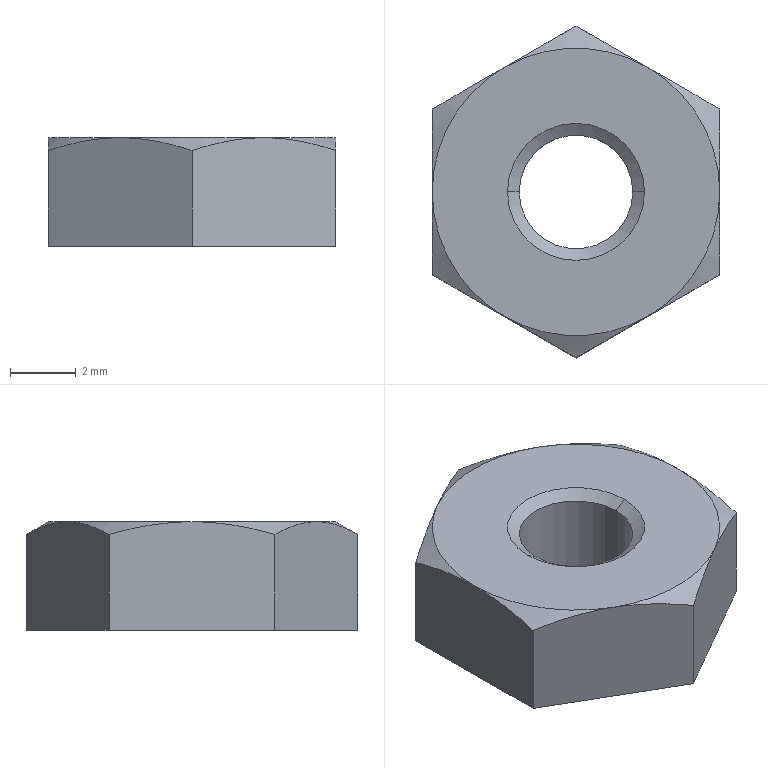Part | SolidWorks | features BaseBody 1 | 1 solid | 22 faces | box 8.738 x 10.089 x 3.302 mm | volume 185.504 mm3 | cone 10 | plane 8 | cylinder 4 | commonest cylinder face diameters 3.454 x2 4.166 x2
STEP:
#1=CARTESIAN_POINT('',(0.,-2.083,-3.302));
#2=VERTEX_POINT('',#1);
#3=CARTESIAN_POINT('',(0.,2.083,-3.302));
#4=VERTEX_POINT('',#3);
#5=CARTESIAN_POINT('',(0.,0.,-3.302));
#6=DIRECTION('',(0.,0.,-1.));
#7=DIRECTION('',(0.,-1.,0.));
#8=AXIS2_PLACEMENT_3D('',#5,#6,#7);
#9=CIRCLE('',#8,2.083);
#10=EDGE_CURVE('',#2,#4,#9,.T.);
#11=ORIENTED_EDGE('',*,*,#10,.T.);
#12=CARTESIAN_POINT('',(0.,2.083,-3.277));
#13=VERTEX_POINT('',#12);
#14=CARTESIAN_POINT('',(0.,2.083,-3.302));
#15=DIRECTION('',(0.,0.,1.));
#16=VECTOR('',#15,1000.);
#17=LINE('',#14,#16);
#18=EDGE_CURVE('',#4,#13,#17,.T.);
#19=ORIENTED_EDGE('',*,*,#18,.T.);
#20=CARTESIAN_POINT('',(-2.083,0.,-3.277));
#21=VERTEX_POINT('',#20);
#22=CARTESIAN_POINT('',(0.,0.,-3.277));
#23=DIRECTION('',(0.,0.,1.));
#24=DIRECTION('',(1.,0.,0.));
#25=AXIS2_PLACEMENT_3D('',#22,#23,#24);
#26=CIRCLE('',#25,2.083);
#27=EDGE_CURVE('',#13,#21,#26,.T.);
#28=ORIENTED_EDGE('',*,*,#27,.T.);
#29=CARTESIAN_POINT('',(0.,-2.083,-3.277));
#30=VERTEX_POINT('',#29);
#31=CARTESIAN_POINT('',(0.,0.,-3.277));
#32=DIRECTION('',(0.,0.,1.));
#33=DIRECTION('',(1.,0.,0.));
#34=AXIS2_PLACEMENT_3D('',#31,#32,#33);
#35=CIRCLE('',#34,2.083);
#36=EDGE_CURVE('',#21,#30,#35,.T.);
#37=ORIENTED_EDGE('',*,*,#36,.T.);
#38=CARTESIAN_POINT('',(0.,-2.083,-3.302));
#39=DIRECTION('',(0.,0.,1.));
#40=VECTOR('',#39,1000.);
#41=LINE('',#38,#40);
#42=EDGE_CURVE('',#2,#30,#41,.T.);
#43=ORIENTED_EDGE('',*,*,#42,.F.);
#44=EDGE_LOOP('',(#11,#19,#28,#37,#43));
#45=FACE_OUTER_BOUND('',#44,.T.);
#46=CARTESIAN_POINT('',(0.,0.,-3.302));
#47=DIRECTION('',(0.,0.,1.));
#48=DIRECTION('',(0.,-1.,0.));
#49=AXIS2_PLACEMENT_3D('',#46,#47,#48);
#50=CYLINDRICAL_SURFACE('',#49,2.083);
#51=ADVANCED_FACE('',(#45),#50,.F.);
#52=CARTESIAN_POINT('',(-1.727,0.,-3.028));
#53=VERTEX_POINT('',#52);
#54=CARTESIAN_POINT('',(1.727,0.,-3.028));
#55=VERTEX_POINT('',#54);
#56=CARTESIAN_POINT('',(0.,0.,-3.028));
#57=DIRECTION('',(0.,0.,1.));
#58=DIRECTION('',(-1.,0.,0.));
#59=AXIS2_PLACEMENT_3D('',#56,#57,#58);
#60=CIRCLE('',#59,1.727);
#61=EDGE_CURVE('',#53,#55,#60,.T.);
#62=ORIENTED_EDGE('',*,*,#61,.T.);
#63=CARTESIAN_POINT('',(2.083,0.,-3.277));
#64=VERTEX_POINT('',#63);
#65=CARTESIAN_POINT('',(1.727,0.,-3.028));
#66=DIRECTION('',(0.8192,0.,-0.5736));
#67=VECTOR('',#66,1000.);
#68=LINE('',#65,#67);
#69=EDGE_CURVE('',#55,#64,#68,.T.);
#70=ORIENTED_EDGE('',*,*,#69,.T.);
#71=CARTESIAN_POINT('',(0.,0.,-3.277));
#72=DIRECTION('',(0.,0.,1.));
#73=DIRECTION('',(1.,0.,0.));
#74=AXIS2_PLACEMENT_3D('',#71,#72,#73);
#75=CIRCLE('',#74,2.083);
#76=EDGE_CURVE('',#30,#64,#75,.T.);
#77=ORIENTED_EDGE('',*,*,#76,.F.);
#78=ORIENTED_EDGE('',*,*,#36,.F.);
#79=CARTESIAN_POINT('',(-1.727,0.,-3.028));
#80=DIRECTION('',(-0.8192,0.,-0.5736));
#81=VECTOR('',#80,1000.);
#82=LINE('',#79,#81);
#83=EDGE_CURVE('',#53,#21,#82,.T.);
#84=ORIENTED_EDGE('',*,*,#83,.F.);
#85=EDGE_LOOP('',(#62,#70,#77,#78,#84));
#86=FACE_OUTER_BOUND('',#85,.T.);
#87=CARTESIAN_POINT('',(0.,0.,-3.028));
#88=DIRECTION('',(0.,0.,-1.));
#89=DIRECTION('',(-1.,0.,0.));
#90=AXIS2_PLACEMENT_3D('',#87,#88,#89);
#91=CONICAL_SURFACE('',#90,1.727,0.9599);
#92=ADVANCED_FACE('',(#86),#91,.F.);
#93=ORIENTED_EDGE('',*,*,#61,.F.);
#94=CARTESIAN_POINT('',(-1.727,0.,-0.249));
#95=VERTEX_POINT('',#94);
#96=CARTESIAN_POINT('',(-1.727,0.,-3.028));
#97=DIRECTION('',(0.,0.,1.));
#98=VECTOR('',#97,1000.);
#99=LINE('',#96,#98);
#100=EDGE_CURVE('',#53,#95,#99,.T.);
#101=ORIENTED_EDGE('',*,*,#100,.T.);
#102=CARTESIAN_POINT('',(1.727,0.,-0.249));
#103=VERTEX_POINT('',#102);
#104=CARTESIAN_POINT('',(0.,0.,-0.249));
#105=DIRECTION('',(0.,0.,1.));
#106=DIRECTION('',(1.,0.,0.));
#107=AXIS2_PLACEMENT_3D('',#104,#105,#106);
#108=CIRCLE('',#107,1.727);
#109=EDGE_CURVE('',#95,#103,#108,.T.);
#110=ORIENTED_EDGE('',*,*,#109,.T.);
#111=CARTESIAN_POINT('',(1.727,0.,-3.028));
#112=DIRECTION('',(0.,0.,1.));
#113=VECTOR('',#112,1000.);
#114=LINE('',#111,#113);
#115=EDGE_CURVE('',#55,#103,#114,.T.);
#116=ORIENTED_EDGE('',*,*,#115,.F.);
#117=EDGE_LOOP('',(#93,#101,#110,#116));
#118=FACE_OUTER_BOUND('',#117,.T.);
#119=CARTESIAN_POINT('',(0.,0.,-3.028));
#120=DIRECTION('',(0.,0.,1.));
#121=DIRECTION('',(1.,0.,0.));
#122=AXIS2_PLACEMENT_3D('',#119,#120,#121);
#123=CYLINDRICAL_SURFACE('',#122,1.727);
#124=ADVANCED_FACE('',(#118),#123,.F.);
#125=ORIENTED_EDGE('',*,*,#109,.F.);
#126=CARTESIAN_POINT('',(-2.083,0.,0.));
#127=VERTEX_POINT('',#126);
#128=CARTESIAN_POINT('',(-1.727,0.,-0.249));
#129=DIRECTION('',(-0.8192,0.,0.5736));
#130=VECTOR('',#129,1000.);
#131=LINE('',#128,#130);
#132=EDGE_CURVE('',#95,#127,#131,.T.);
#133=ORIENTED_EDGE('',*,*,#132,.T.);
#134=CARTESIAN_POINT('',(2.083,0.,0.));
#135=VERTEX_POINT('',#134);
#136=CARTESIAN_POINT('',(0.,0.,0.));
#137=DIRECTION('',(0.,0.,1.));
#138=DIRECTION('',(1.,0.,0.));
#139=AXIS2_PLACEMENT_3D('',#136,#137,#138);
#140=CIRCLE('',#139,2.083);
#141=EDGE_CURVE('',#127,#135,#140,.T.);
#142=ORIENTED_EDGE('',*,*,#141,.T.);
#143=CARTESIAN_POINT('',(1.727,0.,-0.249));
#144=DIRECTION('',(0.8192,0.,0.5736));
#145=VECTOR('',#144,1000.);
#146=LINE('',#143,#145);
#147=EDGE_CURVE('',#103,#135,#146,.T.);
#148=ORIENTED_EDGE('',*,*,#147,.F.);
#149=EDGE_LOOP('',(#125,#133,#142,#148));
#150=FACE_OUTER_BOUND('',#149,.T.);
#151=CARTESIAN_POINT('',(0.,0.,-0.249));
#152=DIRECTION('',(0.,0.,1.));
#153=DIRECTION('',(1.,0.,0.));
#154=AXIS2_PLACEMENT_3D('',#151,#152,#153);
#155=CONICAL_SURFACE('',#154,1.727,0.9599);
#156=ADVANCED_FACE('',(#150),#155,.F.);
#157=ORIENTED_EDGE('',*,*,#18,.F.);
#158=CARTESIAN_POINT('',(0.,0.,-3.302));
#159=DIRECTION('',(0.,0.,-1.));
#160=DIRECTION('',(0.,-1.,0.));
#161=AXIS2_PLACEMENT_3D('',#158,#159,#160);
#162=CIRCLE('',#161,2.083);
#163=EDGE_CURVE('',#4,#2,#162,.T.);
#164=ORIENTED_EDGE('',*,*,#163,.T.);
#165=ORIENTED_EDGE('',*,*,#42,.T.);
#166=ORIENTED_EDGE('',*,*,#76,.T.);
#167=CARTESIAN_POINT('',(0.,0.,-3.277));
#168=DIRECTION('',(0.,0.,1.));
#169=DIRECTION('',(1.,0.,0.));
#170=AXIS2_PLACEMENT_3D('',#167,#168,#169);
#171=CIRCLE('',#170,2.083);
#172=EDGE_CURVE('',#64,#13,#171,.T.);
#173=ORIENTED_EDGE('',*,*,#172,.T.);
#174=EDGE_LOOP('',(#157,#164,#165,#166,#173));
#175=FACE_OUTER_BOUND('',#174,.T.);
#176=CARTESIAN_POINT('',(0.,0.,-3.302));
#177=DIRECTION('',(0.,0.,1.));
#178=DIRECTION('',(0.,-1.,0.));
#179=AXIS2_PLACEMENT_3D('',#176,#177,#178);
#180=CYLINDRICAL_SURFACE('',#179,2.083);
#181=ADVANCED_FACE('',(#175),#180,.F.);
#182=ORIENTED_EDGE('',*,*,#69,.F.);
#183=CARTESIAN_POINT('',(0.,0.,-3.028));
#184=DIRECTION('',(0.,0.,1.));
#185=DIRECTION('',(-1.,0.,0.));
#186=AXIS2_PLACEMENT_3D('',#183,#184,#185);
#187=CIRCLE('',#186,1.727);
#188=EDGE_CURVE('',#55,#53,#187,.T.);
#189=ORIENTED_EDGE('',*,*,#188,.T.);
#190=ORIENTED_EDGE('',*,*,#83,.T.);
#191=ORIENTED_EDGE('',*,*,#27,.F.);
#192=ORIENTED_EDGE('',*,*,#172,.F.);
#193=EDGE_LOOP('',(#182,#189,#190,#191,#192));
#194=FACE_OUTER_BOUND('',#193,.T.);
#195=CARTESIAN_POINT('',(0.,0.,-3.028));
#196=DIRECTION('',(0.,0.,-1.));
#197=DIRECTION('',(-1.,0.,0.));
#198=AXIS2_PLACEMENT_3D('',#195,#196,#197);
#199=CONICAL_SURFACE('',#198,1.727,0.9599);
#200=ADVANCED_FACE('',(#194),#199,.F.);
#201=ORIENTED_EDGE('',*,*,#10,.F.);
#202=ORIENTED_EDGE('',*,*,#163,.F.);
#203=EDGE_LOOP('',(#201,#202));
#204=FACE_BOUND('',#203,.T.);
#205=CARTESIAN_POINT('',(0.,-5.045,-3.302));
#206=VERTEX_POINT('',#205);
#207=CARTESIAN_POINT('',(-4.369,-2.522,-3.302));
#208=VERTEX_POINT('',#207);
#209=CARTESIAN_POINT('',(0.,-5.045,-3.302));
#210=DIRECTION('',(-0.866,0.5,0.));
#211=VECTOR('',#210,1000.);
#212=LINE('',#209,#211);
#213=EDGE_CURVE('',#206,#208,#212,.T.);
#214=ORIENTED_EDGE('',*,*,#213,.T.);
#215=CARTESIAN_POINT('',(-4.369,2.522,-3.302));
#216=VERTEX_POINT('',#215);
#217=CARTESIAN_POINT('',(-4.369,0.,-3.302));
#218=DIRECTION('',(0.,1.,0.));
#219=VECTOR('',#218,1000.);
#220=LINE('',#217,#219);
#221=EDGE_CURVE('',#208,#216,#220,.T.);
#222=ORIENTED_EDGE('',*,*,#221,.T.);
#223=CARTESIAN_POINT('',(0.,5.045,-3.302));
#224=VERTEX_POINT('',#223);
#225=CARTESIAN_POINT('',(-4.369,2.522,-3.302));
#226=DIRECTION('',(0.866,0.5,0.));
#227=VECTOR('',#226,1000.);
#228=LINE('',#225,#227);
#229=EDGE_CURVE('',#216,#224,#228,.T.);
#230=ORIENTED_EDGE('',*,*,#229,.T.);
#231=CARTESIAN_POINT('',(4.369,2.522,-3.302));
#232=VERTEX_POINT('',#231);
#233=CARTESIAN_POINT('',(0.,5.045,-3.302));
#234=DIRECTION('',(0.866,-0.5,0.));
#235=VECTOR('',#234,1000.);
#236=LINE('',#233,#235);
#237=EDGE_CURVE('',#224,#232,#236,.T.);
#238=ORIENTED_EDGE('',*,*,#237,.T.);
#239=CARTESIAN_POINT('',(4.369,-2.522,-3.302));
#240=VERTEX_POINT('',#239);
#241=CARTESIAN_POINT('',(4.369,0.,-3.302));
#242=DIRECTION('',(0.,-1.,0.));
#243=VECTOR('',#242,1000.);
#244=LINE('',#241,#243);
#245=EDGE_CURVE('',#232,#240,#244,.T.);
#246=ORIENTED_EDGE('',*,*,#245,.T.);
#247=CARTESIAN_POINT('',(4.369,-2.522,-3.302));
#248=DIRECTION('',(-0.866,-0.5,0.));
#249=VECTOR('',#248,1000.);
#250=LINE('',#247,#249);
#251=EDGE_CURVE('',#240,#206,#250,.T.);
#252=ORIENTED_EDGE('',*,*,#251,.T.);
#253=EDGE_LOOP('',(#214,#222,#230,#238,#246,#252));
#254=FACE_OUTER_BOUND('',#253,.T.);
#255=CARTESIAN_POINT('',(4.369,-5.105,-3.302));
#256=DIRECTION('',(0.,0.,-1.));
#257=DIRECTION('',(-1.,0.,0.));
#258=AXIS2_PLACEMENT_3D('',#255,#256,#257);
#259=PLANE('',#258);
#260=ADVANCED_FACE('',(#204,#254),#259,.T.);
#261=ORIENTED_EDGE('',*,*,#100,.F.);
#262=ORIENTED_EDGE('',*,*,#188,.F.);
#263=ORIENTED_EDGE('',*,*,#115,.T.);
#264=CARTESIAN_POINT('',(0.,0.,-0.249));
#265=DIRECTION('',(0.,0.,1.));
#266=DIRECTION('',(1.,0.,0.));
#267=AXIS2_PLACEMENT_3D('',#264,#265,#266);
#268=CIRCLE('',#267,1.727);
#269=EDGE_CURVE('',#103,#95,#268,.T.);
#270=ORIENTED_EDGE('',*,*,#269,.T.);
#271=EDGE_LOOP('',(#261,#262,#263,#270));
#272=FACE_OUTER_BOUND('',#271,.T.);
#273=CARTESIAN_POINT('',(0.,0.,-3.028));
#274=DIRECTION('',(0.,0.,1.));
#275=DIRECTION('',(1.,0.,0.));
#276=AXIS2_PLACEMENT_3D('',#273,#274,#275);
#277=CYLINDRICAL_SURFACE('',#276,1.727);
#278=ADVANCED_FACE('',(#272),#277,.F.);
#279=CARTESIAN_POINT('',(-4.369,2.522,-0.3902));
#280=VERTEX_POINT('',#279);
#281=CARTESIAN_POINT('',(-4.369,2.522,-1.641));
#282=DIRECTION('',(0.,0.,-1.));
#283=VECTOR('',#282,1000.);
#284=LINE('',#281,#283);
#285=EDGE_CURVE('',#280,#216,#284,.T.);
#286=ORIENTED_EDGE('',*,*,#285,.T.);
#287=ORIENTED_EDGE('',*,*,#221,.F.);
#288=CARTESIAN_POINT('',(-4.369,-2.522,-0.3902));
#289=VERTEX_POINT('',#288);
#290=CARTESIAN_POINT('',(-4.369,-2.522,-1.641));
#291=DIRECTION('',(0.,0.,1.));
#292=VECTOR('',#291,1000.);
#293=LINE('',#290,#292);
#294=EDGE_CURVE('',#208,#289,#293,.T.);
#295=ORIENTED_EDGE('',*,*,#294,.T.);
#296=CARTESIAN_POINT('',(-4.369,0.,0.));
#297=VERTEX_POINT('',#296);
#298=CARTESIAN_POINT('',(-4.369,-2.522,-0.3902));
#299=CARTESIAN_POINT('',(-4.369,-1.698,-0.1523));
#300=CARTESIAN_POINT('',(-4.369,-0.8609,0.));
#301=CARTESIAN_POINT('',(-4.369,0.,0.));
#302=B_SPLINE_CURVE_WITH_KNOTS('',3,(#298,#299,#300,#301),.UNSPECIFIED.,.F.,.F.,(4,4),(0.,0.002552),.UNSPECIFIED.);
#303=EDGE_CURVE('',#289,#297,#302,.T.);
#304=ORIENTED_EDGE('',*,*,#303,.T.);
#305=CARTESIAN_POINT('',(-4.369,0.,0.));
#306=CARTESIAN_POINT('',(-4.369,0.8609,0.));
#307=CARTESIAN_POINT('',(-4.369,1.698,-0.1523));
#308=CARTESIAN_POINT('',(-4.369,2.522,-0.3902));
#309=B_SPLINE_CURVE_WITH_KNOTS('',3,(#305,#306,#307,#308),.UNSPECIFIED.,.F.,.F.,(4,4),(0.,0.002552),.UNSPECIFIED.);
#310=EDGE_CURVE('',#297,#280,#309,.T.);
#311=ORIENTED_EDGE('',*,*,#310,.T.);
#312=EDGE_LOOP('',(#286,#287,#295,#304,#311));
#313=FACE_OUTER_BOUND('',#312,.T.);
#314=CARTESIAN_POINT('',(-4.369,-2.522,-3.302));
#315=DIRECTION('',(-1.,0.,0.));
#316=DIRECTION('',(0.,0.,1.));
#317=AXIS2_PLACEMENT_3D('',#314,#315,#316);
#318=PLANE('',#317);
#319=ADVANCED_FACE('',(#313),#318,.T.);
#320=ORIENTED_EDGE('',*,*,#294,.F.);
#321=ORIENTED_EDGE('',*,*,#213,.F.);
#322=CARTESIAN_POINT('',(0.,-5.045,-0.3902));
#323=VERTEX_POINT('',#322);
#324=CARTESIAN_POINT('',(0.,-5.045,-1.641));
#325=DIRECTION('',(0.,0.,1.));
#326=VECTOR('',#325,1000.);
#327=LINE('',#324,#326);
#328=EDGE_CURVE('',#206,#323,#327,.T.);
#329=ORIENTED_EDGE('',*,*,#328,.T.);
#330=CARTESIAN_POINT('',(-2.184,-3.783,0.));
#331=VERTEX_POINT('',#330);
#332=CARTESIAN_POINT('',(0.,-5.045,-0.3902));
#333=CARTESIAN_POINT('',(-0.7137,-4.633,-0.1523));
#334=CARTESIAN_POINT('',(-1.439,-4.214,0.));
#335=CARTESIAN_POINT('',(-2.184,-3.783,0.));
#336=B_SPLINE_CURVE_WITH_KNOTS('',3,(#332,#333,#334,#335),.UNSPECIFIED.,.F.,.F.,(4,4),(0.,0.002552),.UNSPECIFIED.);
#337=EDGE_CURVE('',#323,#331,#336,.T.);
#338=ORIENTED_EDGE('',*,*,#337,.T.);
#339=CARTESIAN_POINT('',(-2.184,-3.783,0.));
#340=CARTESIAN_POINT('',(-2.93,-3.353,0.));
#341=CARTESIAN_POINT('',(-3.655,-2.934,-0.1523));
#342=CARTESIAN_POINT('',(-4.369,-2.522,-0.3902));
#343=B_SPLINE_CURVE_WITH_KNOTS('',3,(#339,#340,#341,#342),.UNSPECIFIED.,.F.,.F.,(4,4),(0.,0.002552),.UNSPECIFIED.);
#344=EDGE_CURVE('',#331,#289,#343,.T.);
#345=ORIENTED_EDGE('',*,*,#344,.T.);
#346=EDGE_LOOP('',(#320,#321,#329,#338,#345));
#347=FACE_OUTER_BOUND('',#346,.T.);
#348=CARTESIAN_POINT('',(-4.369,-2.522,-3.302));
#349=DIRECTION('',(-0.5,-0.866,0.));
#350=DIRECTION('',(0.866,-0.5,0.));
#351=AXIS2_PLACEMENT_3D('',#348,#349,#350);
#352=PLANE('',#351);
#353=ADVANCED_FACE('',(#347),#352,.T.);
#354=ORIENTED_EDGE('',*,*,#328,.F.);
#355=ORIENTED_EDGE('',*,*,#251,.F.);
#356=CARTESIAN_POINT('',(4.369,-2.522,-0.3902));
#357=VERTEX_POINT('',#356);
#358=CARTESIAN_POINT('',(4.369,-2.522,-1.641));
#359=DIRECTION('',(0.,0.,1.));
#360=VECTOR('',#359,1000.);
#361=LINE('',#358,#360);
#362=EDGE_CURVE('',#240,#357,#361,.T.);
#363=ORIENTED_EDGE('',*,*,#362,.T.);
#364=CARTESIAN_POINT('',(2.184,-3.783,0.));
#365=VERTEX_POINT('',#364);
#366=CARTESIAN_POINT('',(4.369,-2.522,-0.3902));
#367=CARTESIAN_POINT('',(3.655,-2.934,-0.1523));
#368=CARTESIAN_POINT('',(2.93,-3.353,0.));
#369=CARTESIAN_POINT('',(2.184,-3.783,0.));
#370=B_SPLINE_CURVE_WITH_KNOTS('',3,(#366,#367,#368,#369),.UNSPECIFIED.,.F.,.F.,(4,4),(0.,0.002552),.UNSPECIFIED.);
#371=EDGE_CURVE('',#357,#365,#370,.T.);
#372=ORIENTED_EDGE('',*,*,#371,.T.);
#373=CARTESIAN_POINT('',(2.184,-3.783,0.));
#374=CARTESIAN_POINT('',(1.439,-4.214,0.));
#375=CARTESIAN_POINT('',(0.7137,-4.633,-0.1523));
#376=CARTESIAN_POINT('',(0.,-5.045,-0.3902));
#377=B_SPLINE_CURVE_WITH_KNOTS('',3,(#373,#374,#375,#376),.UNSPECIFIED.,.F.,.F.,(4,4),(0.,0.002552),.UNSPECIFIED.);
#378=EDGE_CURVE('',#365,#323,#377,.T.);
#379=ORIENTED_EDGE('',*,*,#378,.T.);
#380=EDGE_LOOP('',(#354,#355,#363,#372,#379));
#381=FACE_OUTER_BOUND('',#380,.T.);
#382=CARTESIAN_POINT('',(0.,-5.045,-3.302));
#383=DIRECTION('',(0.5,-0.866,0.));
#384=DIRECTION('',(0.866,0.5,0.));
#385=AXIS2_PLACEMENT_3D('',#382,#383,#384);
#386=PLANE('',#385);
#387=ADVANCED_FACE('',(#381),#386,.T.);
#388=ORIENTED_EDGE('',*,*,#362,.F.);
#389=ORIENTED_EDGE('',*,*,#245,.F.);
#390=CARTESIAN_POINT('',(4.369,2.522,-0.3902));
#391=VERTEX_POINT('',#390);
#392=CARTESIAN_POINT('',(4.369,2.522,-1.641));
#393=DIRECTION('',(0.,0.,-1.));
#394=VECTOR('',#393,1000.);
#395=LINE('',#392,#394);
#396=EDGE_CURVE('',#391,#232,#395,.T.);
#397=ORIENTED_EDGE('',*,*,#396,.F.);
#398=CARTESIAN_POINT('',(4.369,-0.000000001,0.));
#399=VERTEX_POINT('',#398);
#400=CARTESIAN_POINT('',(4.369,-0.000000001,0.));
#401=CARTESIAN_POINT('',(4.369,0.8609,0.));
#402=CARTESIAN_POINT('',(4.369,1.698,-0.1523));
#403=CARTESIAN_POINT('',(4.369,2.522,-0.3902));
#404=B_SPLINE_CURVE_WITH_KNOTS('',3,(#400,#401,#402,#403),.UNSPECIFIED.,.F.,.F.,(4,4),(0.,0.002552),.UNSPECIFIED.);
#405=EDGE_CURVE('',#399,#391,#404,.T.);
#406=ORIENTED_EDGE('',*,*,#405,.F.);
#407=CARTESIAN_POINT('',(4.369,-2.522,-0.3902));
#408=CARTESIAN_POINT('',(4.369,-1.698,-0.1523));
#409=CARTESIAN_POINT('',(4.369,-0.8609,0.));
#410=CARTESIAN_POINT('',(4.369,-0.000000001,0.));
#411=B_SPLINE_CURVE_WITH_KNOTS('',3,(#407,#408,#409,#410),.UNSPECIFIED.,.F.,.F.,(4,4),(0.,0.002552),.UNSPECIFIED.);
#412=EDGE_CURVE('',#357,#399,#411,.T.);
#413=ORIENTED_EDGE('',*,*,#412,.F.);
#414=EDGE_LOOP('',(#388,#389,#397,#406,#413));
#415=FACE_OUTER_BOUND('',#414,.T.);
#416=CARTESIAN_POINT('',(4.369,-2.522,-3.302));
#417=DIRECTION('',(-1.,0.,0.));
#418=DIRECTION('',(0.,0.,1.));
#419=AXIS2_PLACEMENT_3D('',#416,#417,#418);
#420=PLANE('',#419);
#421=ADVANCED_FACE('',(#415),#420,.F.);
#422=ORIENTED_EDGE('',*,*,#396,.T.);
#423=ORIENTED_EDGE('',*,*,#237,.F.);
#424=CARTESIAN_POINT('',(0.,5.045,-0.3902));
#425=VERTEX_POINT('',#424);
#426=CARTESIAN_POINT('',(0.,5.045,-1.641));
#427=DIRECTION('',(0.,0.,1.));
#428=VECTOR('',#427,1000.);
#429=LINE('',#426,#428);
#430=EDGE_CURVE('',#224,#425,#429,.T.);
#431=ORIENTED_EDGE('',*,*,#430,.T.);
#432=CARTESIAN_POINT('',(2.184,3.783,0.));
#433=VERTEX_POINT('',#432);
#434=CARTESIAN_POINT('',(0.,5.045,-0.3902));
#435=CARTESIAN_POINT('',(0.7137,4.633,-0.1523));
#436=CARTESIAN_POINT('',(1.439,4.214,0.));
#437=CARTESIAN_POINT('',(2.184,3.783,0.));
#438=B_SPLINE_CURVE_WITH_KNOTS('',3,(#434,#435,#436,#437),.UNSPECIFIED.,.F.,.F.,(4,4),(0.,0.002552),.UNSPECIFIED.);
#439=EDGE_CURVE('',#425,#433,#438,.T.);
#440=ORIENTED_EDGE('',*,*,#439,.T.);
#441=CARTESIAN_POINT('',(2.184,3.783,0.));
#442=CARTESIAN_POINT('',(2.93,3.353,0.));
#443=CARTESIAN_POINT('',(3.655,2.934,-0.1523));
#444=CARTESIAN_POINT('',(4.369,2.522,-0.3902));
#445=B_SPLINE_CURVE_WITH_KNOTS('',3,(#441,#442,#443,#444),.UNSPECIFIED.,.F.,.F.,(4,4),(0.,0.002552),.UNSPECIFIED.);
#446=EDGE_CURVE('',#433,#391,#445,.T.);
#447=ORIENTED_EDGE('',*,*,#446,.T.);
#448=EDGE_LOOP('',(#422,#423,#431,#440,#447));
#449=FACE_OUTER_BOUND('',#448,.T.);
#450=CARTESIAN_POINT('',(4.369,2.522,-3.302));
#451=DIRECTION('',(0.5,0.866,0.));
#452=DIRECTION('',(-0.866,0.5,0.));
#453=AXIS2_PLACEMENT_3D('',#450,#451,#452);
#454=PLANE('',#453);
#455=ADVANCED_FACE('',(#449),#454,.T.);
#456=ORIENTED_EDGE('',*,*,#430,.F.);
#457=ORIENTED_EDGE('',*,*,#229,.F.);
#458=ORIENTED_EDGE('',*,*,#285,.F.);
#459=CARTESIAN_POINT('',(-2.184,3.783,0.));
#460=VERTEX_POINT('',#459);
#461=CARTESIAN_POINT('',(-4.369,2.522,-0.3902));
#462=CARTESIAN_POINT('',(-3.655,2.934,-0.1523));
#463=CARTESIAN_POINT('',(-2.93,3.353,0.));
#464=CARTESIAN_POINT('',(-2.184,3.783,0.));
#465=B_SPLINE_CURVE_WITH_KNOTS('',3,(#461,#462,#463,#464),.UNSPECIFIED.,.F.,.F.,(4,4),(0.,0.002552),.UNSPECIFIED.);
#466=EDGE_CURVE('',#280,#460,#465,.T.);
#467=ORIENTED_EDGE('',*,*,#466,.T.);
#468=CARTESIAN_POINT('',(-2.184,3.783,0.));
#469=CARTESIAN_POINT('',(-1.439,4.214,0.));
#470=CARTESIAN_POINT('',(-0.7137,4.633,-0.1523));
#471=CARTESIAN_POINT('',(0.,5.045,-0.3902));
#472=B_SPLINE_CURVE_WITH_KNOTS('',3,(#468,#469,#470,#471),.UNSPECIFIED.,.F.,.F.,(4,4),(0.,0.002552),.UNSPECIFIED.);
#473=EDGE_CURVE('',#460,#425,#472,.T.);
#474=ORIENTED_EDGE('',*,*,#473,.T.);
#475=EDGE_LOOP('',(#456,#457,#458,#467,#474));
#476=FACE_OUTER_BOUND('',#475,.T.);
#477=CARTESIAN_POINT('',(0.,5.045,-3.302));
#478=DIRECTION('',(-0.5,0.866,0.));
#479=DIRECTION('',(-0.866,-0.5,0.));
#480=AXIS2_PLACEMENT_3D('',#477,#478,#479);
#481=PLANE('',#480);
#482=ADVANCED_FACE('',(#476),#481,.T.);
#483=ORIENTED_EDGE('',*,*,#132,.F.);
#484=ORIENTED_EDGE('',*,*,#269,.F.);
#485=ORIENTED_EDGE('',*,*,#147,.T.);
#486=CARTESIAN_POINT('',(0.,0.,0.));
#487=DIRECTION('',(0.,0.,1.));
#488=DIRECTION('',(1.,0.,0.));
#489=AXIS2_PLACEMENT_3D('',#486,#487,#488);
#490=CIRCLE('',#489,2.083);
#491=EDGE_CURVE('',#135,#127,#490,.T.);
#492=ORIENTED_EDGE('',*,*,#491,.T.);
#493=EDGE_LOOP('',(#483,#484,#485,#492));
#494=FACE_OUTER_BOUND('',#493,.T.);
#495=CARTESIAN_POINT('',(0.,0.,-0.249));
#496=DIRECTION('',(0.,0.,1.));
#497=DIRECTION('',(1.,0.,0.));
#498=AXIS2_PLACEMENT_3D('',#495,#496,#497);
#499=CONICAL_SURFACE('',#498,1.727,0.9599);
#500=ADVANCED_FACE('',(#494),#499,.F.);
#501=CARTESIAN_POINT('',(0.,0.,0.));
#502=DIRECTION('',(0.,0.,1.));
#503=DIRECTION('',(-1.,0.,0.));
#504=AXIS2_PLACEMENT_3D('',#501,#502,#503);
#505=CIRCLE('',#504,4.369);
#506=EDGE_CURVE('',#460,#297,#505,.T.);
#507=ORIENTED_EDGE('',*,*,#506,.F.);
#508=ORIENTED_EDGE('',*,*,#466,.F.);
#509=ORIENTED_EDGE('',*,*,#310,.F.);
#510=EDGE_LOOP('',(#507,#508,#509));
#511=FACE_OUTER_BOUND('',#510,.T.);
#512=CARTESIAN_POINT('',(0.,0.,0.));
#513=DIRECTION('',(0.,0.,-1.));
#514=DIRECTION('',(-1.,0.,0.));
#515=AXIS2_PLACEMENT_3D('',#512,#513,#514);
#516=CONICAL_SURFACE('',#515,4.369,1.047);
#517=ADVANCED_FACE('',(#511),#516,.T.);
#518=ORIENTED_EDGE('',*,*,#303,.F.);
#519=ORIENTED_EDGE('',*,*,#344,.F.);
#520=CARTESIAN_POINT('',(0.,0.,0.));
#521=DIRECTION('',(0.,0.,1.));
#522=DIRECTION('',(-1.,0.,0.));
#523=AXIS2_PLACEMENT_3D('',#520,#521,#522);
#524=CIRCLE('',#523,4.369);
#525=EDGE_CURVE('',#297,#331,#524,.T.);
#526=ORIENTED_EDGE('',*,*,#525,.F.);
#527=EDGE_LOOP('',(#518,#519,#526));
#528=FACE_OUTER_BOUND('',#527,.T.);
#529=CARTESIAN_POINT('',(0.,0.,0.));
#530=DIRECTION('',(0.,0.,-1.));
#531=DIRECTION('',(-1.,0.,0.));
#532=AXIS2_PLACEMENT_3D('',#529,#530,#531);
#533=CONICAL_SURFACE('',#532,4.369,1.047);
#534=ADVANCED_FACE('',(#528),#533,.T.);
#535=ORIENTED_EDGE('',*,*,#337,.F.);
#536=ORIENTED_EDGE('',*,*,#378,.F.);
#537=CARTESIAN_POINT('',(0.,0.,0.));
#538=DIRECTION('',(0.,0.,1.));
#539=DIRECTION('',(-1.,0.,0.));
#540=AXIS2_PLACEMENT_3D('',#537,#538,#539);
#541=CIRCLE('',#540,4.369);
#542=EDGE_CURVE('',#331,#365,#541,.T.);
#543=ORIENTED_EDGE('',*,*,#542,.F.);
#544=EDGE_LOOP('',(#535,#536,#543));
#545=FACE_OUTER_BOUND('',#544,.T.);
#546=CARTESIAN_POINT('',(0.,0.,0.));
#547=DIRECTION('',(0.,0.,-1.));
#548=DIRECTION('',(-1.,0.,0.));
#549=AXIS2_PLACEMENT_3D('',#546,#547,#548);
#550=CONICAL_SURFACE('',#549,4.369,1.047);
#551=ADVANCED_FACE('',(#545),#550,.T.);
#552=CARTESIAN_POINT('',(0.,0.,0.));
#553=DIRECTION('',(0.,0.,1.));
#554=DIRECTION('',(-1.,0.,0.));
#555=AXIS2_PLACEMENT_3D('',#552,#553,#554);
#556=CIRCLE('',#555,4.369);
#557=EDGE_CURVE('',#365,#399,#556,.T.);
#558=ORIENTED_EDGE('',*,*,#557,.F.);
#559=ORIENTED_EDGE('',*,*,#371,.F.);
#560=ORIENTED_EDGE('',*,*,#412,.T.);
#561=EDGE_LOOP('',(#558,#559,#560));
#562=FACE_OUTER_BOUND('',#561,.T.);
#563=CARTESIAN_POINT('',(0.,0.,0.));
#564=DIRECTION('',(0.,0.,-1.));
#565=DIRECTION('',(-1.,0.,0.));
#566=AXIS2_PLACEMENT_3D('',#563,#564,#565);
#567=CONICAL_SURFACE('',#566,4.369,1.047);
#568=ADVANCED_FACE('',(#562),#567,.T.);
#569=ORIENTED_EDGE('',*,*,#405,.T.);
#570=ORIENTED_EDGE('',*,*,#446,.F.);
#571=CARTESIAN_POINT('',(0.,0.,0.));
#572=DIRECTION('',(0.,0.,1.));
#573=DIRECTION('',(-1.,0.,0.));
#574=AXIS2_PLACEMENT_3D('',#571,#572,#573);
#575=CIRCLE('',#574,4.369);
#576=EDGE_CURVE('',#399,#433,#575,.T.);
#577=ORIENTED_EDGE('',*,*,#576,.F.);
#578=EDGE_LOOP('',(#569,#570,#577));
#579=FACE_OUTER_BOUND('',#578,.T.);
#580=CARTESIAN_POINT('',(0.,0.,0.));
#581=DIRECTION('',(0.,0.,-1.));
#582=DIRECTION('',(-1.,0.,0.));
#583=AXIS2_PLACEMENT_3D('',#580,#581,#582);
#584=CONICAL_SURFACE('',#583,4.369,1.047);
#585=ADVANCED_FACE('',(#579),#584,.T.);
#586=ORIENTED_EDGE('',*,*,#439,.F.);
#587=ORIENTED_EDGE('',*,*,#473,.F.);
#588=CARTESIAN_POINT('',(0.,0.,0.));
#589=DIRECTION('',(0.,0.,1.));
#590=DIRECTION('',(-1.,0.,0.));
#591=AXIS2_PLACEMENT_3D('',#588,#589,#590);
#592=CIRCLE('',#591,4.369);
#593=EDGE_CURVE('',#433,#460,#592,.T.);
#594=ORIENTED_EDGE('',*,*,#593,.F.);
#595=EDGE_LOOP('',(#586,#587,#594));
#596=FACE_OUTER_BOUND('',#595,.T.);
#597=CARTESIAN_POINT('',(0.,0.,0.));
#598=DIRECTION('',(0.,0.,-1.));
#599=DIRECTION('',(-1.,0.,0.));
#600=AXIS2_PLACEMENT_3D('',#597,#598,#599);
#601=CONICAL_SURFACE('',#600,4.369,1.047);
#602=ADVANCED_FACE('',(#596),#601,.T.);
#603=ORIENTED_EDGE('',*,*,#491,.F.);
#604=ORIENTED_EDGE('',*,*,#141,.F.);
#605=EDGE_LOOP('',(#603,#604));
#606=FACE_BOUND('',#605,.T.);
#607=ORIENTED_EDGE('',*,*,#525,.T.);
#608=ORIENTED_EDGE('',*,*,#542,.T.);
#609=ORIENTED_EDGE('',*,*,#557,.T.);
#610=ORIENTED_EDGE('',*,*,#576,.T.);
#611=ORIENTED_EDGE('',*,*,#593,.T.);
#612=ORIENTED_EDGE('',*,*,#506,.T.);
#613=EDGE_LOOP('',(#607,#608,#609,#610,#611,#612));
#614=FACE_OUTER_BOUND('',#613,.T.);
#615=CARTESIAN_POINT('',(4.421,-4.421,0.));
#616=DIRECTION('',(0.,0.,-1.));
#617=DIRECTION('',(-1.,0.,0.));
#618=AXIS2_PLACEMENT_3D('',#615,#616,#617);
#619=PLANE('',#618);
#620=ADVANCED_FACE('',(#606,#614),#619,.F.);
#621=CLOSED_SHELL('',(#51,#92,#124,#156,#181,#200,#260,#278,#319,#353,#387,#421,#455,#482,#500,#517,#534,#551,#568,#585,#602,#620));
#622=MANIFOLD_SOLID_BREP('',#621);
#623=CARTESIAN_POINT('',(0.,0.,0.));
#624=DIRECTION('',(0.,0.,1.));
#625=DIRECTION('',(1.,0.,0.));
#626=AXIS2_PLACEMENT_3D('',#623,#624,#625);
#627=(LENGTH_UNIT()NAMED_UNIT(*)SI_UNIT(.MILLI.,.METRE.));
#628=UNCERTAINTY_MEASURE_WITH_UNIT(LENGTH_MEASURE(0.00001),#627,'','');
#629=(NAMED_UNIT(*)PLANE_ANGLE_UNIT()SI_UNIT($,.RADIAN.));
#630=(NAMED_UNIT(*)SI_UNIT($,.STERADIAN.)SOLID_ANGLE_UNIT());
#631=(GEOMETRIC_REPRESENTATION_CONTEXT(3)GLOBAL_UNCERTAINTY_ASSIGNED_CONTEXT((#628))GLOBAL_UNIT_ASSIGNED_CONTEXT((#627,#629,#630))REPRESENTATION_CONTEXT('',''));
#632=ADVANCED_BREP_SHAPE_REPRESENTATION('',(#622,#626),#631);